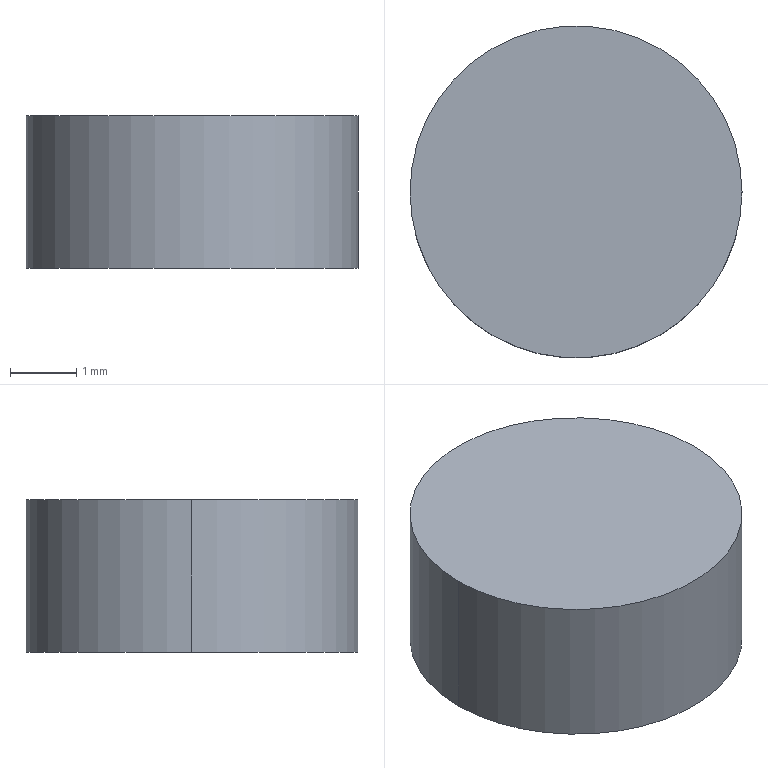Part | STEP file | ASND-0110-Body 1-5 | 1 solid | 4 faces | box 5 x 5 x 2.3 mm | volume 45.16 mm3 | cylinder 2 | plane 2 | commonest cylinder face diameters 5 x2
STEP:
#1=CARTESIAN_POINT('',(0.,0.,0.));
#2=DIRECTION('',(0.,0.,1.));
#3=DIRECTION('',(1.,0.,0.));
#4=AXIS2_PLACEMENT_3D('',#1,#2,#3);
#5=CARTESIAN_POINT('',(2.5,0.,0.));
#6=VERTEX_POINT('',#5);
#7=CARTESIAN_POINT('',(-2.5,0.,0.));
#8=VERTEX_POINT('',#7);
#9=CARTESIAN_POINT('',(0.,0.,0.));
#10=DIRECTION('',(0.,0.,-1.));
#11=DIRECTION('',(-1.,0.,0.));
#12=AXIS2_PLACEMENT_3D('',#9,#10,#11);
#13=CIRCLE('',#12,2.5);
#14=CARTESIAN_POINT('',(0.,0.,0.));
#15=DIRECTION('',(0.,0.,1.));
#16=DIRECTION('',(-1.,0.,0.));
#17=AXIS2_PLACEMENT_3D('',#14,#15,#16);
#18=CYLINDRICAL_SURFACE('',#17,2.5);
#19=CARTESIAN_POINT('',(6.283,0.));
#20=DIRECTION('',(-1.,0.));
#21=VECTOR('',#20,1.);
#22=LINE('',#19,#21);
#23=(GEOMETRIC_REPRESENTATION_CONTEXT(2)PARAMETRIC_REPRESENTATION_CONTEXT()REPRESENTATION_CONTEXT('',''));
#24=DEFINITIONAL_REPRESENTATION('',(#22),#23);
#25=PCURVE('',#18,#24);
#26=CARTESIAN_POINT('',(0.,0.,0.));
#27=DIRECTION('',(0.,0.,-1.));
#28=DIRECTION('',(0.7071,0.7071,0.));
#29=AXIS2_PLACEMENT_3D('',#26,#27,#28);
#30=PLANE('',#29);
#31=CARTESIAN_POINT('',(0.,0.));
#32=DIRECTION('',(-0.7071,-0.7071));
#33=AXIS2_PLACEMENT_2D('',#31,#32);
#34=CIRCLE('',#33,2.5);
#35=(GEOMETRIC_REPRESENTATION_CONTEXT(2)PARAMETRIC_REPRESENTATION_CONTEXT()REPRESENTATION_CONTEXT('',''));
#36=DEFINITIONAL_REPRESENTATION('',(#34),#35);
#37=PCURVE('',#30,#36);
#38=SURFACE_CURVE('',#13,(#25,#37),.PCURVE_S1.);
#39=EDGE_CURVE('',#6,#8,#38,.T.);
#40=ORIENTED_EDGE('',*,*,#39,.F.);
#41=CARTESIAN_POINT('',(2.5,0.,2.3));
#42=VERTEX_POINT('',#41);
#43=CARTESIAN_POINT('',(2.5,0.,0.));
#44=DIRECTION('',(0.,0.,1.));
#45=VECTOR('',#44,1.);
#46=LINE('',#43,#45);
#47=CARTESIAN_POINT('',(3.142,0.));
#48=DIRECTION('',(0.,1.));
#49=VECTOR('',#48,1.);
#50=LINE('',#47,#49);
#51=(GEOMETRIC_REPRESENTATION_CONTEXT(2)PARAMETRIC_REPRESENTATION_CONTEXT()REPRESENTATION_CONTEXT('',''));
#52=DEFINITIONAL_REPRESENTATION('',(#50),#51);
#53=PCURVE('',#18,#52);
#54=CARTESIAN_POINT('',(0.,0.,0.));
#55=DIRECTION('',(0.,0.,1.));
#56=DIRECTION('',(-1.,0.,0.));
#57=AXIS2_PLACEMENT_3D('',#54,#55,#56);
#58=CYLINDRICAL_SURFACE('',#57,2.5);
#59=CARTESIAN_POINT('',(3.142,0.));
#60=DIRECTION('',(0.,1.));
#61=VECTOR('',#60,1.);
#62=LINE('',#59,#61);
#63=(GEOMETRIC_REPRESENTATION_CONTEXT(2)PARAMETRIC_REPRESENTATION_CONTEXT()REPRESENTATION_CONTEXT('',''));
#64=DEFINITIONAL_REPRESENTATION('',(#62),#63);
#65=PCURVE('',#58,#64);
#66=SURFACE_CURVE('',#46,(#53,#65),.PCURVE_S1.);
#67=EDGE_CURVE('',#6,#42,#66,.T.);
#68=ORIENTED_EDGE('',*,*,#67,.T.);
#69=CARTESIAN_POINT('',(-2.5,0.,2.3));
#70=VERTEX_POINT('',#69);
#71=CARTESIAN_POINT('',(0.,0.,2.3));
#72=DIRECTION('',(0.,0.,-1.));
#73=DIRECTION('',(-1.,0.,0.));
#74=AXIS2_PLACEMENT_3D('',#71,#72,#73);
#75=CIRCLE('',#74,2.5);
#76=CARTESIAN_POINT('',(6.283,2.3));
#77=DIRECTION('',(-1.,0.));
#78=VECTOR('',#77,1.);
#79=LINE('',#76,#78);
#80=(GEOMETRIC_REPRESENTATION_CONTEXT(2)PARAMETRIC_REPRESENTATION_CONTEXT()REPRESENTATION_CONTEXT('',''));
#81=DEFINITIONAL_REPRESENTATION('',(#79),#80);
#82=PCURVE('',#18,#81);
#83=CARTESIAN_POINT('',(0.,0.,2.3));
#84=DIRECTION('',(0.,0.,-1.));
#85=DIRECTION('',(0.7071,0.7071,0.));
#86=AXIS2_PLACEMENT_3D('',#83,#84,#85);
#87=PLANE('',#86);
#88=CARTESIAN_POINT('',(0.,0.));
#89=DIRECTION('',(-0.7071,-0.7071));
#90=AXIS2_PLACEMENT_2D('',#88,#89);
#91=CIRCLE('',#90,2.5);
#92=(GEOMETRIC_REPRESENTATION_CONTEXT(2)PARAMETRIC_REPRESENTATION_CONTEXT()REPRESENTATION_CONTEXT('',''));
#93=DEFINITIONAL_REPRESENTATION('',(#91),#92);
#94=PCURVE('',#87,#93);
#95=SURFACE_CURVE('',#75,(#82,#94),.PCURVE_S1.);
#96=EDGE_CURVE('',#42,#70,#95,.T.);
#97=ORIENTED_EDGE('',*,*,#96,.T.);
#98=CARTESIAN_POINT('',(-2.5,0.,0.));
#99=DIRECTION('',(0.,0.,1.));
#100=VECTOR('',#99,1.);
#101=LINE('',#98,#100);
#102=CARTESIAN_POINT('',(0.,0.));
#103=DIRECTION('',(0.,1.));
#104=VECTOR('',#103,1.);
#105=LINE('',#102,#104);
#106=(GEOMETRIC_REPRESENTATION_CONTEXT(2)PARAMETRIC_REPRESENTATION_CONTEXT()REPRESENTATION_CONTEXT('',''));
#107=DEFINITIONAL_REPRESENTATION('',(#105),#106);
#108=PCURVE('',#18,#107);
#109=CARTESIAN_POINT('',(6.283,0.));
#110=DIRECTION('',(0.,1.));
#111=VECTOR('',#110,1.);
#112=LINE('',#109,#111);
#113=(GEOMETRIC_REPRESENTATION_CONTEXT(2)PARAMETRIC_REPRESENTATION_CONTEXT()REPRESENTATION_CONTEXT('',''));
#114=DEFINITIONAL_REPRESENTATION('',(#112),#113);
#115=PCURVE('',#58,#114);
#116=SURFACE_CURVE('',#101,(#108,#115),.PCURVE_S1.);
#117=EDGE_CURVE('',#8,#70,#116,.T.);
#118=ORIENTED_EDGE('',*,*,#117,.F.);
#119=EDGE_LOOP('',(#40,#68,#97,#118));
#120=FACE_BOUND('',#119,.T.);
#121=ADVANCED_FACE('',(#120),#18,.T.);
#122=ORIENTED_EDGE('',*,*,#67,.F.);
#123=CARTESIAN_POINT('',(0.,0.,0.));
#124=DIRECTION('',(0.,0.,-1.));
#125=DIRECTION('',(-1.,0.,0.));
#126=AXIS2_PLACEMENT_3D('',#123,#124,#125);
#127=CIRCLE('',#126,2.5);
#128=CARTESIAN_POINT('',(6.283,0.));
#129=DIRECTION('',(-1.,0.));
#130=VECTOR('',#129,1.);
#131=LINE('',#128,#130);
#132=(GEOMETRIC_REPRESENTATION_CONTEXT(2)PARAMETRIC_REPRESENTATION_CONTEXT()REPRESENTATION_CONTEXT('',''));
#133=DEFINITIONAL_REPRESENTATION('',(#131),#132);
#134=PCURVE('',#58,#133);
#135=CARTESIAN_POINT('',(0.,0.));
#136=DIRECTION('',(-0.7071,-0.7071));
#137=AXIS2_PLACEMENT_2D('',#135,#136);
#138=CIRCLE('',#137,2.5);
#139=(GEOMETRIC_REPRESENTATION_CONTEXT(2)PARAMETRIC_REPRESENTATION_CONTEXT()REPRESENTATION_CONTEXT('',''));
#140=DEFINITIONAL_REPRESENTATION('',(#138),#139);
#141=PCURVE('',#30,#140);
#142=SURFACE_CURVE('',#127,(#134,#141),.PCURVE_S1.);
#143=EDGE_CURVE('',#8,#6,#142,.T.);
#144=ORIENTED_EDGE('',*,*,#143,.F.);
#145=ORIENTED_EDGE('',*,*,#117,.T.);
#146=CARTESIAN_POINT('',(0.,0.,2.3));
#147=DIRECTION('',(0.,0.,-1.));
#148=DIRECTION('',(-1.,0.,0.));
#149=AXIS2_PLACEMENT_3D('',#146,#147,#148);
#150=CIRCLE('',#149,2.5);
#151=CARTESIAN_POINT('',(6.283,2.3));
#152=DIRECTION('',(-1.,0.));
#153=VECTOR('',#152,1.);
#154=LINE('',#151,#153);
#155=(GEOMETRIC_REPRESENTATION_CONTEXT(2)PARAMETRIC_REPRESENTATION_CONTEXT()REPRESENTATION_CONTEXT('',''));
#156=DEFINITIONAL_REPRESENTATION('',(#154),#155);
#157=PCURVE('',#58,#156);
#158=CARTESIAN_POINT('',(0.,0.));
#159=DIRECTION('',(-0.7071,-0.7071));
#160=AXIS2_PLACEMENT_2D('',#158,#159);
#161=CIRCLE('',#160,2.5);
#162=(GEOMETRIC_REPRESENTATION_CONTEXT(2)PARAMETRIC_REPRESENTATION_CONTEXT()REPRESENTATION_CONTEXT('',''));
#163=DEFINITIONAL_REPRESENTATION('',(#161),#162);
#164=PCURVE('',#87,#163);
#165=SURFACE_CURVE('',#150,(#157,#164),.PCURVE_S1.);
#166=EDGE_CURVE('',#70,#42,#165,.T.);
#167=ORIENTED_EDGE('',*,*,#166,.T.);
#168=EDGE_LOOP('',(#122,#144,#145,#167));
#169=FACE_BOUND('',#168,.T.);
#170=ADVANCED_FACE('',(#169),#58,.T.);
#171=ORIENTED_EDGE('',*,*,#166,.F.);
#172=ORIENTED_EDGE('',*,*,#96,.F.);
#173=EDGE_LOOP('',(#171,#172));
#174=FACE_BOUND('',#173,.T.);
#175=ADVANCED_FACE('',(#174),#87,.F.);
#176=ORIENTED_EDGE('',*,*,#143,.T.);
#177=ORIENTED_EDGE('',*,*,#39,.T.);
#178=EDGE_LOOP('',(#176,#177));
#179=FACE_BOUND('',#178,.T.);
#180=ADVANCED_FACE('',(#179),#30,.T.);
#181=CLOSED_SHELL('',(#121,#170,#175,#180));
#182=MANIFOLD_SOLID_BREP('',#181);
#183=(LENGTH_UNIT()NAMED_UNIT(*)SI_UNIT(.MILLI.,.METRE.));
#184=UNCERTAINTY_MEASURE_WITH_UNIT(LENGTH_MEASURE(0.0000001),#183,'','');
#185=(NAMED_UNIT(*)PLANE_ANGLE_UNIT()SI_UNIT($,.RADIAN.));
#186=(NAMED_UNIT(*)SI_UNIT($,.STERADIAN.)SOLID_ANGLE_UNIT());
#187=(GEOMETRIC_REPRESENTATION_CONTEXT(3)GLOBAL_UNCERTAINTY_ASSIGNED_CONTEXT((#184))GLOBAL_UNIT_ASSIGNED_CONTEXT((#183,#185,#186))REPRESENTATION_CONTEXT('',''));
#188=ADVANCED_BREP_SHAPE_REPRESENTATION('',(#4,#182),#187);